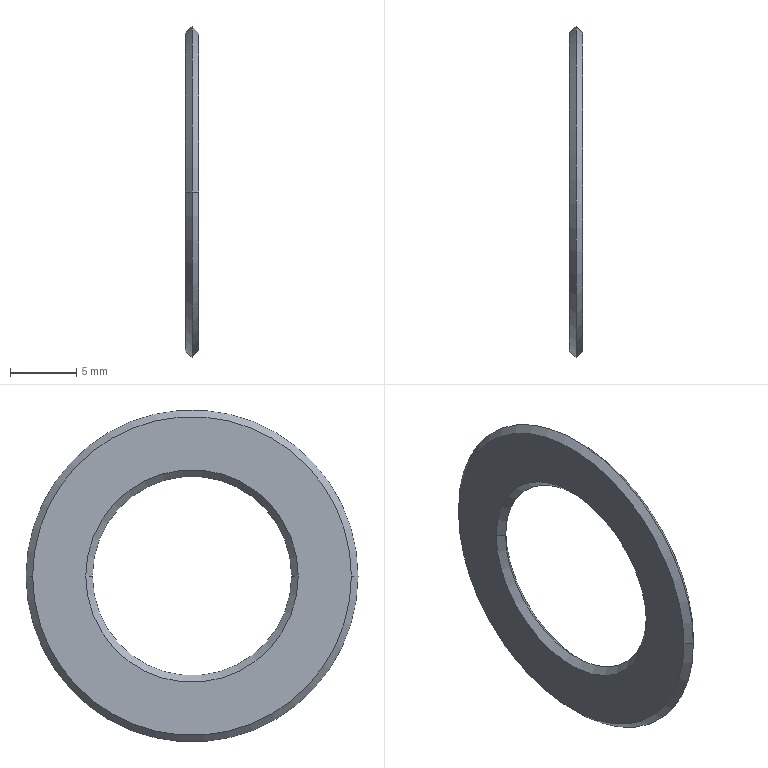Part | STEP file | 0217_005_WSSS25-15-1 | 1 solid | 10 faces | box 1 x 25 x 25 mm | volume 282.743 mm3 | cone 8 | plane 2
STEP:
#1=CARTESIAN_POINT('',(0.,0.,0.));
#2=DIRECTION('',(0.,0.,1.));
#3=DIRECTION('',(1.,0.,0.));
#4=AXIS2_PLACEMENT_3D('',#1,#2,#3);
#5=CARTESIAN_POINT('',(1.,12.,0.));
#6=VERTEX_POINT('',#5);
#7=CARTESIAN_POINT('',(1.,-12.,0.));
#8=VERTEX_POINT('',#7);
#9=CARTESIAN_POINT('',(1.,0.,0.));
#10=DIRECTION('',(1.,0.,0.));
#11=DIRECTION('',(0.,-1.,0.));
#12=AXIS2_PLACEMENT_3D('',#9,#10,#11);
#13=CIRCLE('',#12,12.);
#14=CARTESIAN_POINT('',(0.5,0.,0.));
#15=DIRECTION('',(-1.,0.,0.));
#16=DIRECTION('',(0.,-1.,0.));
#17=AXIS2_PLACEMENT_3D('',#14,#15,#16);
#18=CONICAL_SURFACE('',#17,12.5,0.7854);
#19=CARTESIAN_POINT('',(6.283,-0.5));
#20=DIRECTION('',(-1.,0.));
#21=VECTOR('',#20,1.);
#22=LINE('',#19,#21);
#23=(GEOMETRIC_REPRESENTATION_CONTEXT(2)PARAMETRIC_REPRESENTATION_CONTEXT()REPRESENTATION_CONTEXT('',''));
#24=DEFINITIONAL_REPRESENTATION('',(#22),#23);
#25=PCURVE('',#18,#24);
#26=CARTESIAN_POINT('',(1.,-10.,0.));
#27=DIRECTION('',(1.,0.,0.));
#28=DIRECTION('',(0.,1.,0.));
#29=AXIS2_PLACEMENT_3D('',#26,#27,#28);
#30=PLANE('',#29);
#31=CARTESIAN_POINT('',(10.,0.));
#32=DIRECTION('',(-1.,0.));
#33=AXIS2_PLACEMENT_2D('',#31,#32);
#34=CIRCLE('',#33,12.);
#35=(GEOMETRIC_REPRESENTATION_CONTEXT(2)PARAMETRIC_REPRESENTATION_CONTEXT()REPRESENTATION_CONTEXT('',''));
#36=DEFINITIONAL_REPRESENTATION('',(#34),#35);
#37=PCURVE('',#30,#36);
#38=SURFACE_CURVE('',#13,(#25,#37),.PCURVE_S1.);
#39=EDGE_CURVE('',#6,#8,#38,.T.);
#40=ORIENTED_EDGE('',*,*,#39,.F.);
#41=CARTESIAN_POINT('',(0.5,12.5,0.));
#42=VERTEX_POINT('',#41);
#43=CARTESIAN_POINT('',(0.5,12.5,0.));
#44=DIRECTION('',(-0.7071,0.7071,0.));
#45=VECTOR('',#44,1.);
#46=LINE('',#43,#45);
#47=CARTESIAN_POINT('',(3.142,0.));
#48=DIRECTION('',(0.,1.));
#49=VECTOR('',#48,1.);
#50=LINE('',#47,#49);
#51=(GEOMETRIC_REPRESENTATION_CONTEXT(2)PARAMETRIC_REPRESENTATION_CONTEXT()REPRESENTATION_CONTEXT('',''));
#52=DEFINITIONAL_REPRESENTATION('',(#50),#51);
#53=PCURVE('',#18,#52);
#54=CARTESIAN_POINT('',(0.5,0.,0.));
#55=DIRECTION('',(-1.,0.,0.));
#56=DIRECTION('',(0.,-1.,0.));
#57=AXIS2_PLACEMENT_3D('',#54,#55,#56);
#58=CONICAL_SURFACE('',#57,12.5,0.7854);
#59=CARTESIAN_POINT('',(3.142,0.));
#60=DIRECTION('',(0.,1.));
#61=VECTOR('',#60,1.);
#62=LINE('',#59,#61);
#63=(GEOMETRIC_REPRESENTATION_CONTEXT(2)PARAMETRIC_REPRESENTATION_CONTEXT()REPRESENTATION_CONTEXT('',''));
#64=DEFINITIONAL_REPRESENTATION('',(#62),#63);
#65=PCURVE('',#58,#64);
#66=SURFACE_CURVE('',#46,(#53,#65),.PCURVE_S1.);
#67=EDGE_CURVE('',#6,#42,#66,.T.);
#68=ORIENTED_EDGE('',*,*,#67,.T.);
#69=CARTESIAN_POINT('',(0.5,-12.5,0.));
#70=VERTEX_POINT('',#69);
#71=CARTESIAN_POINT('',(0.5,0.,0.));
#72=DIRECTION('',(1.,0.,0.));
#73=DIRECTION('',(0.,-1.,0.));
#74=AXIS2_PLACEMENT_3D('',#71,#72,#73);
#75=CIRCLE('',#74,12.5);
#76=CARTESIAN_POINT('',(6.283,0.));
#77=DIRECTION('',(-1.,0.));
#78=VECTOR('',#77,1.);
#79=LINE('',#76,#78);
#80=(GEOMETRIC_REPRESENTATION_CONTEXT(2)PARAMETRIC_REPRESENTATION_CONTEXT()REPRESENTATION_CONTEXT('',''));
#81=DEFINITIONAL_REPRESENTATION('',(#79),#80);
#82=PCURVE('',#18,#81);
#83=CARTESIAN_POINT('',(0.5,0.,0.));
#84=DIRECTION('',(1.,0.,0.));
#85=DIRECTION('',(0.,1.,0.));
#86=AXIS2_PLACEMENT_3D('',#83,#84,#85);
#87=CONICAL_SURFACE('',#86,12.5,0.7854);
#88=CARTESIAN_POINT('',(-3.142,0.));
#89=DIRECTION('',(1.,0.));
#90=VECTOR('',#89,1.);
#91=LINE('',#88,#90);
#92=(GEOMETRIC_REPRESENTATION_CONTEXT(2)PARAMETRIC_REPRESENTATION_CONTEXT()REPRESENTATION_CONTEXT('',''));
#93=DEFINITIONAL_REPRESENTATION('',(#91),#92);
#94=PCURVE('',#87,#93);
#95=SURFACE_CURVE('',#75,(#82,#94),.PCURVE_S1.);
#96=EDGE_CURVE('',#42,#70,#95,.T.);
#97=ORIENTED_EDGE('',*,*,#96,.T.);
#98=CARTESIAN_POINT('',(0.5,-12.5,0.));
#99=DIRECTION('',(-0.7071,-0.7071,0.));
#100=VECTOR('',#99,1.);
#101=LINE('',#98,#100);
#102=CARTESIAN_POINT('',(0.,0.));
#103=DIRECTION('',(0.,1.));
#104=VECTOR('',#103,1.);
#105=LINE('',#102,#104);
#106=(GEOMETRIC_REPRESENTATION_CONTEXT(2)PARAMETRIC_REPRESENTATION_CONTEXT()REPRESENTATION_CONTEXT('',''));
#107=DEFINITIONAL_REPRESENTATION('',(#105),#106);
#108=PCURVE('',#18,#107);
#109=CARTESIAN_POINT('',(6.283,0.));
#110=DIRECTION('',(0.,1.));
#111=VECTOR('',#110,1.);
#112=LINE('',#109,#111);
#113=(GEOMETRIC_REPRESENTATION_CONTEXT(2)PARAMETRIC_REPRESENTATION_CONTEXT()REPRESENTATION_CONTEXT('',''));
#114=DEFINITIONAL_REPRESENTATION('',(#112),#113);
#115=PCURVE('',#58,#114);
#116=SURFACE_CURVE('',#101,(#108,#115),.PCURVE_S1.);
#117=EDGE_CURVE('',#8,#70,#116,.T.);
#118=ORIENTED_EDGE('',*,*,#117,.F.);
#119=EDGE_LOOP('',(#40,#68,#97,#118));
#120=FACE_BOUND('',#119,.T.);
#121=ADVANCED_FACE('',(#120),#18,.T.);
#122=CARTESIAN_POINT('',(0.5,7.5,0.));
#123=VERTEX_POINT('',#122);
#124=CARTESIAN_POINT('',(1.,8.,0.));
#125=VERTEX_POINT('',#124);
#126=CARTESIAN_POINT('',(1.,8.,0.));
#127=DIRECTION('',(0.7071,0.7071,0.));
#128=VECTOR('',#127,1.);
#129=LINE('',#126,#128);
#130=CARTESIAN_POINT('',(1.,0.,0.));
#131=DIRECTION('',(1.,0.,0.));
#132=DIRECTION('',(0.,1.,0.));
#133=AXIS2_PLACEMENT_3D('',#130,#131,#132);
#134=CONICAL_SURFACE('',#133,8.,0.7854);
#135=CARTESIAN_POINT('',(6.283,0.));
#136=DIRECTION('',(0.,1.));
#137=VECTOR('',#136,1.);
#138=LINE('',#135,#137);
#139=(GEOMETRIC_REPRESENTATION_CONTEXT(2)PARAMETRIC_REPRESENTATION_CONTEXT()REPRESENTATION_CONTEXT('',''));
#140=DEFINITIONAL_REPRESENTATION('',(#138),#139);
#141=PCURVE('',#134,#140);
#142=CARTESIAN_POINT('',(1.,0.,0.));
#143=DIRECTION('',(1.,0.,0.));
#144=DIRECTION('',(0.,1.,0.));
#145=AXIS2_PLACEMENT_3D('',#142,#143,#144);
#146=CONICAL_SURFACE('',#145,8.,0.7854);
#147=CARTESIAN_POINT('',(0.,0.));
#148=DIRECTION('',(0.,1.));
#149=VECTOR('',#148,1.);
#150=LINE('',#147,#149);
#151=(GEOMETRIC_REPRESENTATION_CONTEXT(2)PARAMETRIC_REPRESENTATION_CONTEXT()REPRESENTATION_CONTEXT('',''));
#152=DEFINITIONAL_REPRESENTATION('',(#150),#151);
#153=PCURVE('',#146,#152);
#154=SURFACE_CURVE('',#129,(#141,#153),.PCURVE_S1.);
#155=EDGE_CURVE('',#123,#125,#154,.T.);
#156=ORIENTED_EDGE('',*,*,#155,.T.);
#157=CARTESIAN_POINT('',(1.,-8.,0.));
#158=VERTEX_POINT('',#157);
#159=CARTESIAN_POINT('',(1.,0.,0.));
#160=DIRECTION('',(-1.,0.,0.));
#161=DIRECTION('',(0.,1.,0.));
#162=AXIS2_PLACEMENT_3D('',#159,#160,#161);
#163=CIRCLE('',#162,8.);
#164=CARTESIAN_POINT('',(6.283,0.));
#165=DIRECTION('',(-1.,0.));
#166=VECTOR('',#165,1.);
#167=LINE('',#164,#166);
#168=(GEOMETRIC_REPRESENTATION_CONTEXT(2)PARAMETRIC_REPRESENTATION_CONTEXT()REPRESENTATION_CONTEXT('',''));
#169=DEFINITIONAL_REPRESENTATION('',(#167),#168);
#170=PCURVE('',#134,#169);
#171=CARTESIAN_POINT('',(18.,0.));
#172=CARTESIAN_POINT('',(18.,-13.856));
#173=CARTESIAN_POINT('',(6.,-6.928));
#174=CARTESIAN_POINT('',(-6.,0.));
#175=CARTESIAN_POINT('',(6.,6.928));
#176=CARTESIAN_POINT('',(18.,13.856));
#177=CARTESIAN_POINT('',(18.,0.));
#178=(BOUNDED_CURVE()B_SPLINE_CURVE(2,(#171,#172,#173,#174,#175,#176,#177),.UNSPECIFIED.,.T.,.F.)B_SPLINE_CURVE_WITH_KNOTS((1,2,2,2,2,1),(-2.094,0.,2.094,4.189,6.283,8.378),.UNSPECIFIED.)CURVE()GEOMETRIC_REPRESENTATION_ITEM()RATIONAL_B_SPLINE_CURVE((1.,0.5,1.,0.5,1.,0.5,1.))REPRESENTATION_ITEM(''));
#179=(GEOMETRIC_REPRESENTATION_CONTEXT(2)PARAMETRIC_REPRESENTATION_CONTEXT()REPRESENTATION_CONTEXT('',''));
#180=DEFINITIONAL_REPRESENTATION('',(#178),#179);
#181=PCURVE('',#30,#180);
#182=SURFACE_CURVE('',#163,(#170,#181),.PCURVE_S1.);
#183=EDGE_CURVE('',#125,#158,#182,.T.);
#184=ORIENTED_EDGE('',*,*,#183,.T.);
#185=CARTESIAN_POINT('',(0.5,-7.5,0.));
#186=VERTEX_POINT('',#185);
#187=CARTESIAN_POINT('',(1.,-8.,0.));
#188=DIRECTION('',(0.7071,-0.7071,0.));
#189=VECTOR('',#188,1.);
#190=LINE('',#187,#189);
#191=CARTESIAN_POINT('',(3.142,0.));
#192=DIRECTION('',(0.,1.));
#193=VECTOR('',#192,1.);
#194=LINE('',#191,#193);
#195=(GEOMETRIC_REPRESENTATION_CONTEXT(2)PARAMETRIC_REPRESENTATION_CONTEXT()REPRESENTATION_CONTEXT('',''));
#196=DEFINITIONAL_REPRESENTATION('',(#194),#195);
#197=PCURVE('',#134,#196);
#198=CARTESIAN_POINT('',(3.142,0.));
#199=DIRECTION('',(0.,1.));
#200=VECTOR('',#199,1.);
#201=LINE('',#198,#200);
#202=(GEOMETRIC_REPRESENTATION_CONTEXT(2)PARAMETRIC_REPRESENTATION_CONTEXT()REPRESENTATION_CONTEXT('',''));
#203=DEFINITIONAL_REPRESENTATION('',(#201),#202);
#204=PCURVE('',#146,#203);
#205=SURFACE_CURVE('',#190,(#197,#204),.PCURVE_S1.);
#206=EDGE_CURVE('',#186,#158,#205,.T.);
#207=ORIENTED_EDGE('',*,*,#206,.F.);
#208=CARTESIAN_POINT('',(0.5,0.,0.));
#209=DIRECTION('',(1.,0.,0.));
#210=DIRECTION('',(0.,-1.,0.));
#211=AXIS2_PLACEMENT_3D('',#208,#209,#210);
#212=CIRCLE('',#211,7.5);
#213=CARTESIAN_POINT('',(3.142,-0.5));
#214=DIRECTION('',(1.,0.));
#215=VECTOR('',#214,1.);
#216=LINE('',#213,#215);
#217=(GEOMETRIC_REPRESENTATION_CONTEXT(2)PARAMETRIC_REPRESENTATION_CONTEXT()REPRESENTATION_CONTEXT('',''));
#218=DEFINITIONAL_REPRESENTATION('',(#216),#217);
#219=PCURVE('',#134,#218);
#220=CARTESIAN_POINT('',(0.,0.,0.));
#221=DIRECTION('',(-1.,0.,0.));
#222=DIRECTION('',(0.,-1.,0.));
#223=AXIS2_PLACEMENT_3D('',#220,#221,#222);
#224=CONICAL_SURFACE('',#223,8.,0.7854);
#225=CARTESIAN_POINT('',(6.283,-0.5));
#226=DIRECTION('',(-1.,0.));
#227=VECTOR('',#226,1.);
#228=LINE('',#225,#227);
#229=(GEOMETRIC_REPRESENTATION_CONTEXT(2)PARAMETRIC_REPRESENTATION_CONTEXT()REPRESENTATION_CONTEXT('',''));
#230=DEFINITIONAL_REPRESENTATION('',(#228),#229);
#231=PCURVE('',#224,#230);
#232=SURFACE_CURVE('',#212,(#219,#231),.PCURVE_S1.);
#233=EDGE_CURVE('',#186,#123,#232,.T.);
#234=ORIENTED_EDGE('',*,*,#233,.T.);
#235=EDGE_LOOP('',(#156,#184,#207,#234));
#236=FACE_BOUND('',#235,.F.);
#237=ADVANCED_FACE('',(#236),#134,.F.);
#238=CARTESIAN_POINT('',(0.,12.,0.));
#239=VERTEX_POINT('',#238);
#240=CARTESIAN_POINT('',(0.,-12.,0.));
#241=VERTEX_POINT('',#240);
#242=CARTESIAN_POINT('',(0.,0.,0.));
#243=DIRECTION('',(1.,0.,0.));
#244=DIRECTION('',(0.,1.,0.));
#245=AXIS2_PLACEMENT_3D('',#242,#243,#244);
#246=CIRCLE('',#245,12.);
#247=CARTESIAN_POINT('',(0.,-0.5));
#248=DIRECTION('',(1.,0.));
#249=VECTOR('',#248,1.);
#250=LINE('',#247,#249);
#251=(GEOMETRIC_REPRESENTATION_CONTEXT(2)PARAMETRIC_REPRESENTATION_CONTEXT()REPRESENTATION_CONTEXT('',''));
#252=DEFINITIONAL_REPRESENTATION('',(#250),#251);
#253=PCURVE('',#87,#252);
#254=CARTESIAN_POINT('',(0.,-10.,0.));
#255=DIRECTION('',(-1.,0.,0.));
#256=DIRECTION('',(0.,-1.,0.));
#257=AXIS2_PLACEMENT_3D('',#254,#255,#256);
#258=PLANE('',#257);
#259=CARTESIAN_POINT('',(-22.,0.));
#260=CARTESIAN_POINT('',(-22.,20.785));
#261=CARTESIAN_POINT('',(-4.,10.392));
#262=CARTESIAN_POINT('',(14.,0.));
#263=CARTESIAN_POINT('',(-4.,-10.392));
#264=CARTESIAN_POINT('',(-22.,-20.785));
#265=CARTESIAN_POINT('',(-22.,0.));
#266=(BOUNDED_CURVE()B_SPLINE_CURVE(2,(#259,#260,#261,#262,#263,#264,#265),.UNSPECIFIED.,.T.,.F.)B_SPLINE_CURVE_WITH_KNOTS((1,2,2,2,2,1),(-2.094,0.,2.094,4.189,6.283,8.378),.UNSPECIFIED.)CURVE()GEOMETRIC_REPRESENTATION_ITEM()RATIONAL_B_SPLINE_CURVE((1.,0.5,1.,0.5,1.,0.5,1.))REPRESENTATION_ITEM(''));
#267=(GEOMETRIC_REPRESENTATION_CONTEXT(2)PARAMETRIC_REPRESENTATION_CONTEXT()REPRESENTATION_CONTEXT('',''));
#268=DEFINITIONAL_REPRESENTATION('',(#266),#267);
#269=PCURVE('',#258,#268);
#270=SURFACE_CURVE('',#246,(#253,#269),.PCURVE_S1.);
#271=EDGE_CURVE('',#239,#241,#270,.T.);
#272=ORIENTED_EDGE('',*,*,#271,.T.);
#273=CARTESIAN_POINT('',(0.5,-12.5,0.));
#274=DIRECTION('',(0.7071,-0.7071,0.));
#275=VECTOR('',#274,1.);
#276=LINE('',#273,#275);
#277=CARTESIAN_POINT('',(3.142,0.));
#278=DIRECTION('',(0.,1.));
#279=VECTOR('',#278,1.);
#280=LINE('',#277,#279);
#281=(GEOMETRIC_REPRESENTATION_CONTEXT(2)PARAMETRIC_REPRESENTATION_CONTEXT()REPRESENTATION_CONTEXT('',''));
#282=DEFINITIONAL_REPRESENTATION('',(#280),#281);
#283=PCURVE('',#87,#282);
#284=CARTESIAN_POINT('',(0.5,0.,0.));
#285=DIRECTION('',(1.,0.,0.));
#286=DIRECTION('',(0.,1.,0.));
#287=AXIS2_PLACEMENT_3D('',#284,#285,#286);
#288=CONICAL_SURFACE('',#287,12.5,0.7854);
#289=CARTESIAN_POINT('',(3.142,0.));
#290=DIRECTION('',(0.,1.));
#291=VECTOR('',#290,1.);
#292=LINE('',#289,#291);
#293=(GEOMETRIC_REPRESENTATION_CONTEXT(2)PARAMETRIC_REPRESENTATION_CONTEXT()REPRESENTATION_CONTEXT('',''));
#294=DEFINITIONAL_REPRESENTATION('',(#292),#293);
#295=PCURVE('',#288,#294);
#296=SURFACE_CURVE('',#276,(#283,#295),.PCURVE_S1.);
#297=EDGE_CURVE('',#241,#70,#296,.T.);
#298=ORIENTED_EDGE('',*,*,#297,.T.);
#299=ORIENTED_EDGE('',*,*,#96,.F.);
#300=CARTESIAN_POINT('',(0.5,12.5,0.));
#301=DIRECTION('',(0.7071,0.7071,0.));
#302=VECTOR('',#301,1.);
#303=LINE('',#300,#302);
#304=CARTESIAN_POINT('',(0.,0.));
#305=DIRECTION('',(0.,1.));
#306=VECTOR('',#305,1.);
#307=LINE('',#304,#306);
#308=(GEOMETRIC_REPRESENTATION_CONTEXT(2)PARAMETRIC_REPRESENTATION_CONTEXT()REPRESENTATION_CONTEXT('',''));
#309=DEFINITIONAL_REPRESENTATION('',(#307),#308);
#310=PCURVE('',#87,#309);
#311=CARTESIAN_POINT('',(6.283,0.));
#312=DIRECTION('',(0.,1.));
#313=VECTOR('',#312,1.);
#314=LINE('',#311,#313);
#315=(GEOMETRIC_REPRESENTATION_CONTEXT(2)PARAMETRIC_REPRESENTATION_CONTEXT()REPRESENTATION_CONTEXT('',''));
#316=DEFINITIONAL_REPRESENTATION('',(#314),#315);
#317=PCURVE('',#288,#316);
#318=SURFACE_CURVE('',#303,(#310,#317),.PCURVE_S1.);
#319=EDGE_CURVE('',#239,#42,#318,.T.);
#320=ORIENTED_EDGE('',*,*,#319,.F.);
#321=EDGE_LOOP('',(#272,#298,#299,#320));
#322=FACE_BOUND('',#321,.T.);
#323=ADVANCED_FACE('',(#322),#87,.T.);
#324=CARTESIAN_POINT('',(0.,-8.,0.));
#325=VERTEX_POINT('',#324);
#326=CARTESIAN_POINT('',(0.,-8.,0.));
#327=DIRECTION('',(-0.7071,-0.7071,0.));
#328=VECTOR('',#327,1.);
#329=LINE('',#326,#328);
#330=CARTESIAN_POINT('',(6.283,0.));
#331=DIRECTION('',(0.,1.));
#332=VECTOR('',#331,1.);
#333=LINE('',#330,#332);
#334=(GEOMETRIC_REPRESENTATION_CONTEXT(2)PARAMETRIC_REPRESENTATION_CONTEXT()REPRESENTATION_CONTEXT('',''));
#335=DEFINITIONAL_REPRESENTATION('',(#333),#334);
#336=PCURVE('',#224,#335);
#337=CARTESIAN_POINT('',(0.,0.,0.));
#338=DIRECTION('',(-1.,0.,0.));
#339=DIRECTION('',(0.,-1.,0.));
#340=AXIS2_PLACEMENT_3D('',#337,#338,#339);
#341=CONICAL_SURFACE('',#340,8.,0.7854);
#342=CARTESIAN_POINT('',(0.,0.));
#343=DIRECTION('',(0.,1.));
#344=VECTOR('',#343,1.);
#345=LINE('',#342,#344);
#346=(GEOMETRIC_REPRESENTATION_CONTEXT(2)PARAMETRIC_REPRESENTATION_CONTEXT()REPRESENTATION_CONTEXT('',''));
#347=DEFINITIONAL_REPRESENTATION('',(#345),#346);
#348=PCURVE('',#341,#347);
#349=SURFACE_CURVE('',#329,(#336,#348),.PCURVE_S1.);
#350=EDGE_CURVE('',#186,#325,#349,.T.);
#351=ORIENTED_EDGE('',*,*,#350,.T.);
#352=CARTESIAN_POINT('',(0.,8.,0.));
#353=VERTEX_POINT('',#352);
#354=CARTESIAN_POINT('',(0.,0.,0.));
#355=DIRECTION('',(1.,0.,0.));
#356=DIRECTION('',(0.,-1.,0.));
#357=AXIS2_PLACEMENT_3D('',#354,#355,#356);
#358=CIRCLE('',#357,8.);
#359=CARTESIAN_POINT('',(6.283,0.));
#360=DIRECTION('',(-1.,0.));
#361=VECTOR('',#360,1.);
#362=LINE('',#359,#361);
#363=(GEOMETRIC_REPRESENTATION_CONTEXT(2)PARAMETRIC_REPRESENTATION_CONTEXT()REPRESENTATION_CONTEXT('',''));
#364=DEFINITIONAL_REPRESENTATION('',(#362),#363);
#365=PCURVE('',#224,#364);
#366=CARTESIAN_POINT('',(-2.,0.));
#367=CARTESIAN_POINT('',(-2.,-13.856));
#368=CARTESIAN_POINT('',(-14.,-6.928));
#369=CARTESIAN_POINT('',(-26.,0.));
#370=CARTESIAN_POINT('',(-14.,6.928));
#371=CARTESIAN_POINT('',(-2.,13.856));
#372=CARTESIAN_POINT('',(-2.,0.));
#373=(BOUNDED_CURVE()B_SPLINE_CURVE(2,(#366,#367,#368,#369,#370,#371,#372),.UNSPECIFIED.,.T.,.F.)B_SPLINE_CURVE_WITH_KNOTS((1,2,2,2,2,1),(-2.094,0.,2.094,4.189,6.283,8.378),.UNSPECIFIED.)CURVE()GEOMETRIC_REPRESENTATION_ITEM()RATIONAL_B_SPLINE_CURVE((1.,0.5,1.,0.5,1.,0.5,1.))REPRESENTATION_ITEM(''));
#374=(GEOMETRIC_REPRESENTATION_CONTEXT(2)PARAMETRIC_REPRESENTATION_CONTEXT()REPRESENTATION_CONTEXT('',''));
#375=DEFINITIONAL_REPRESENTATION('',(#373),#374);
#376=PCURVE('',#258,#375);
#377=SURFACE_CURVE('',#358,(#365,#376),.PCURVE_S1.);
#378=EDGE_CURVE('',#325,#353,#377,.T.);
#379=ORIENTED_EDGE('',*,*,#378,.T.);
#380=CARTESIAN_POINT('',(0.,8.,0.));
#381=DIRECTION('',(-0.7071,0.7071,0.));
#382=VECTOR('',#381,1.);
#383=LINE('',#380,#382);
#384=CARTESIAN_POINT('',(3.142,0.));
#385=DIRECTION('',(0.,1.));
#386=VECTOR('',#385,1.);
#387=LINE('',#384,#386);
#388=(GEOMETRIC_REPRESENTATION_CONTEXT(2)PARAMETRIC_REPRESENTATION_CONTEXT()REPRESENTATION_CONTEXT('',''));
#389=DEFINITIONAL_REPRESENTATION('',(#387),#388);
#390=PCURVE('',#224,#389);
#391=CARTESIAN_POINT('',(3.142,0.));
#392=DIRECTION('',(0.,1.));
#393=VECTOR('',#392,1.);
#394=LINE('',#391,#393);
#395=(GEOMETRIC_REPRESENTATION_CONTEXT(2)PARAMETRIC_REPRESENTATION_CONTEXT()REPRESENTATION_CONTEXT('',''));
#396=DEFINITIONAL_REPRESENTATION('',(#394),#395);
#397=PCURVE('',#341,#396);
#398=SURFACE_CURVE('',#383,(#390,#397),.PCURVE_S1.);
#399=EDGE_CURVE('',#123,#353,#398,.T.);
#400=ORIENTED_EDGE('',*,*,#399,.F.);
#401=ORIENTED_EDGE('',*,*,#233,.F.);
#402=EDGE_LOOP('',(#351,#379,#400,#401));
#403=FACE_BOUND('',#402,.F.);
#404=ADVANCED_FACE('',(#403),#224,.F.);
#405=CARTESIAN_POINT('',(1.,0.,0.));
#406=DIRECTION('',(1.,0.,0.));
#407=DIRECTION('',(0.,-1.,0.));
#408=AXIS2_PLACEMENT_3D('',#405,#406,#407);
#409=CIRCLE('',#408,12.);
#410=CARTESIAN_POINT('',(10.,0.));
#411=DIRECTION('',(-1.,0.));
#412=AXIS2_PLACEMENT_2D('',#410,#411);
#413=CIRCLE('',#412,12.);
#414=(GEOMETRIC_REPRESENTATION_CONTEXT(2)PARAMETRIC_REPRESENTATION_CONTEXT()REPRESENTATION_CONTEXT('',''));
#415=DEFINITIONAL_REPRESENTATION('',(#413),#414);
#416=PCURVE('',#30,#415);
#417=CARTESIAN_POINT('',(6.283,-0.5));
#418=DIRECTION('',(-1.,0.));
#419=VECTOR('',#418,1.);
#420=LINE('',#417,#419);
#421=(GEOMETRIC_REPRESENTATION_CONTEXT(2)PARAMETRIC_REPRESENTATION_CONTEXT()REPRESENTATION_CONTEXT('',''));
#422=DEFINITIONAL_REPRESENTATION('',(#420),#421);
#423=PCURVE('',#58,#422);
#424=SURFACE_CURVE('',#409,(#416,#423),.PCURVE_S1.);
#425=EDGE_CURVE('',#8,#6,#424,.T.);
#426=ORIENTED_EDGE('',*,*,#425,.T.);
#427=ORIENTED_EDGE('',*,*,#39,.T.);
#428=EDGE_LOOP('',(#426,#427));
#429=FACE_BOUND('',#428,.T.);
#430=ORIENTED_EDGE('',*,*,#183,.T.);
#431=CARTESIAN_POINT('',(1.,0.,0.));
#432=DIRECTION('',(-1.,0.,0.));
#433=DIRECTION('',(0.,1.,0.));
#434=AXIS2_PLACEMENT_3D('',#431,#432,#433);
#435=CIRCLE('',#434,8.);
#436=CARTESIAN_POINT('',(18.,0.));
#437=CARTESIAN_POINT('',(18.,-13.856));
#438=CARTESIAN_POINT('',(6.,-6.928));
#439=CARTESIAN_POINT('',(-6.,0.));
#440=CARTESIAN_POINT('',(6.,6.928));
#441=CARTESIAN_POINT('',(18.,13.856));
#442=CARTESIAN_POINT('',(18.,0.));
#443=(BOUNDED_CURVE()B_SPLINE_CURVE(2,(#436,#437,#438,#439,#440,#441,#442),.UNSPECIFIED.,.T.,.F.)B_SPLINE_CURVE_WITH_KNOTS((1,2,2,2,2,1),(-2.094,0.,2.094,4.189,6.283,8.378),.UNSPECIFIED.)CURVE()GEOMETRIC_REPRESENTATION_ITEM()RATIONAL_B_SPLINE_CURVE((1.,0.5,1.,0.5,1.,0.5,1.))REPRESENTATION_ITEM(''));
#444=(GEOMETRIC_REPRESENTATION_CONTEXT(2)PARAMETRIC_REPRESENTATION_CONTEXT()REPRESENTATION_CONTEXT('',''));
#445=DEFINITIONAL_REPRESENTATION('',(#443),#444);
#446=PCURVE('',#30,#445);
#447=CARTESIAN_POINT('',(6.283,0.));
#448=DIRECTION('',(-1.,0.));
#449=VECTOR('',#448,1.);
#450=LINE('',#447,#449);
#451=(GEOMETRIC_REPRESENTATION_CONTEXT(2)PARAMETRIC_REPRESENTATION_CONTEXT()REPRESENTATION_CONTEXT('',''));
#452=DEFINITIONAL_REPRESENTATION('',(#450),#451);
#453=PCURVE('',#146,#452);
#454=SURFACE_CURVE('',#435,(#446,#453),.PCURVE_S1.);
#455=EDGE_CURVE('',#158,#125,#454,.T.);
#456=ORIENTED_EDGE('',*,*,#455,.T.);
#457=EDGE_LOOP('',(#430,#456));
#458=FACE_BOUND('',#457,.T.);
#459=ADVANCED_FACE('',(#429,#458),#30,.T.);
#460=ORIENTED_EDGE('',*,*,#67,.F.);
#461=ORIENTED_EDGE('',*,*,#425,.F.);
#462=ORIENTED_EDGE('',*,*,#117,.T.);
#463=CARTESIAN_POINT('',(0.5,0.,0.));
#464=DIRECTION('',(1.,0.,0.));
#465=DIRECTION('',(0.,-1.,0.));
#466=AXIS2_PLACEMENT_3D('',#463,#464,#465);
#467=CIRCLE('',#466,12.5);
#468=CARTESIAN_POINT('',(6.283,0.));
#469=DIRECTION('',(-1.,0.));
#470=VECTOR('',#469,1.);
#471=LINE('',#468,#470);
#472=(GEOMETRIC_REPRESENTATION_CONTEXT(2)PARAMETRIC_REPRESENTATION_CONTEXT()REPRESENTATION_CONTEXT('',''));
#473=DEFINITIONAL_REPRESENTATION('',(#471),#472);
#474=PCURVE('',#58,#473);
#475=CARTESIAN_POINT('',(3.142,0.));
#476=DIRECTION('',(1.,0.));
#477=VECTOR('',#476,1.);
#478=LINE('',#475,#477);
#479=(GEOMETRIC_REPRESENTATION_CONTEXT(2)PARAMETRIC_REPRESENTATION_CONTEXT()REPRESENTATION_CONTEXT('',''));
#480=DEFINITIONAL_REPRESENTATION('',(#478),#479);
#481=PCURVE('',#288,#480);
#482=SURFACE_CURVE('',#467,(#474,#481),.PCURVE_S1.);
#483=EDGE_CURVE('',#70,#42,#482,.T.);
#484=ORIENTED_EDGE('',*,*,#483,.T.);
#485=EDGE_LOOP('',(#460,#461,#462,#484));
#486=FACE_BOUND('',#485,.T.);
#487=ADVANCED_FACE('',(#486),#58,.T.);
#488=ORIENTED_EDGE('',*,*,#455,.T.);
#489=ORIENTED_EDGE('',*,*,#155,.F.);
#490=CARTESIAN_POINT('',(0.5,0.,0.));
#491=DIRECTION('',(1.,0.,0.));
#492=DIRECTION('',(0.,-1.,0.));
#493=AXIS2_PLACEMENT_3D('',#490,#491,#492);
#494=CIRCLE('',#493,7.5);
#495=CARTESIAN_POINT('',(-3.142,-0.5));
#496=DIRECTION('',(1.,0.));
#497=VECTOR('',#496,1.);
#498=LINE('',#495,#497);
#499=(GEOMETRIC_REPRESENTATION_CONTEXT(2)PARAMETRIC_REPRESENTATION_CONTEXT()REPRESENTATION_CONTEXT('',''));
#500=DEFINITIONAL_REPRESENTATION('',(#498),#499);
#501=PCURVE('',#146,#500);
#502=CARTESIAN_POINT('',(6.283,-0.5));
#503=DIRECTION('',(-1.,0.));
#504=VECTOR('',#503,1.);
#505=LINE('',#502,#504);
#506=(GEOMETRIC_REPRESENTATION_CONTEXT(2)PARAMETRIC_REPRESENTATION_CONTEXT()REPRESENTATION_CONTEXT('',''));
#507=DEFINITIONAL_REPRESENTATION('',(#505),#506);
#508=PCURVE('',#341,#507);
#509=SURFACE_CURVE('',#494,(#501,#508),.PCURVE_S1.);
#510=EDGE_CURVE('',#123,#186,#509,.T.);
#511=ORIENTED_EDGE('',*,*,#510,.T.);
#512=ORIENTED_EDGE('',*,*,#206,.T.);
#513=EDGE_LOOP('',(#488,#489,#511,#512));
#514=FACE_BOUND('',#513,.F.);
#515=ADVANCED_FACE('',(#514),#146,.F.);
#516=ORIENTED_EDGE('',*,*,#297,.F.);
#517=CARTESIAN_POINT('',(0.,0.,0.));
#518=DIRECTION('',(1.,0.,0.));
#519=DIRECTION('',(0.,1.,0.));
#520=AXIS2_PLACEMENT_3D('',#517,#518,#519);
#521=CIRCLE('',#520,12.);
#522=CARTESIAN_POINT('',(0.,-0.5));
#523=DIRECTION('',(1.,0.));
#524=VECTOR('',#523,1.);
#525=LINE('',#522,#524);
#526=(GEOMETRIC_REPRESENTATION_CONTEXT(2)PARAMETRIC_REPRESENTATION_CONTEXT()REPRESENTATION_CONTEXT('',''));
#527=DEFINITIONAL_REPRESENTATION('',(#525),#526);
#528=PCURVE('',#288,#527);
#529=CARTESIAN_POINT('',(-22.,0.));
#530=CARTESIAN_POINT('',(-22.,20.785));
#531=CARTESIAN_POINT('',(-4.,10.392));
#532=CARTESIAN_POINT('',(14.,0.));
#533=CARTESIAN_POINT('',(-4.,-10.392));
#534=CARTESIAN_POINT('',(-22.,-20.785));
#535=CARTESIAN_POINT('',(-22.,0.));
#536=(BOUNDED_CURVE()B_SPLINE_CURVE(2,(#529,#530,#531,#532,#533,#534,#535),.UNSPECIFIED.,.T.,.F.)B_SPLINE_CURVE_WITH_KNOTS((1,2,2,2,2,1),(-2.094,0.,2.094,4.189,6.283,8.378),.UNSPECIFIED.)CURVE()GEOMETRIC_REPRESENTATION_ITEM()RATIONAL_B_SPLINE_CURVE((1.,0.5,1.,0.5,1.,0.5,1.))REPRESENTATION_ITEM(''));
#537=(GEOMETRIC_REPRESENTATION_CONTEXT(2)PARAMETRIC_REPRESENTATION_CONTEXT()REPRESENTATION_CONTEXT('',''));
#538=DEFINITIONAL_REPRESENTATION('',(#536),#537);
#539=PCURVE('',#258,#538);
#540=SURFACE_CURVE('',#521,(#528,#539),.PCURVE_S1.);
#541=EDGE_CURVE('',#241,#239,#540,.T.);
#542=ORIENTED_EDGE('',*,*,#541,.T.);
#543=ORIENTED_EDGE('',*,*,#319,.T.);
#544=ORIENTED_EDGE('',*,*,#483,.F.);
#545=EDGE_LOOP('',(#516,#542,#543,#544));
#546=FACE_BOUND('',#545,.T.);
#547=ADVANCED_FACE('',(#546),#288,.T.);
#548=CARTESIAN_POINT('',(0.,0.,0.));
#549=DIRECTION('',(1.,0.,0.));
#550=DIRECTION('',(0.,-1.,0.));
#551=AXIS2_PLACEMENT_3D('',#548,#549,#550);
#552=CIRCLE('',#551,8.);
#553=CARTESIAN_POINT('',(6.283,0.));
#554=DIRECTION('',(-1.,0.));
#555=VECTOR('',#554,1.);
#556=LINE('',#553,#555);
#557=(GEOMETRIC_REPRESENTATION_CONTEXT(2)PARAMETRIC_REPRESENTATION_CONTEXT()REPRESENTATION_CONTEXT('',''));
#558=DEFINITIONAL_REPRESENTATION('',(#556),#557);
#559=PCURVE('',#341,#558);
#560=CARTESIAN_POINT('',(-2.,0.));
#561=CARTESIAN_POINT('',(-2.,-13.856));
#562=CARTESIAN_POINT('',(-14.,-6.928));
#563=CARTESIAN_POINT('',(-26.,0.));
#564=CARTESIAN_POINT('',(-14.,6.928));
#565=CARTESIAN_POINT('',(-2.,13.856));
#566=CARTESIAN_POINT('',(-2.,0.));
#567=(BOUNDED_CURVE()B_SPLINE_CURVE(2,(#560,#561,#562,#563,#564,#565,#566),.UNSPECIFIED.,.T.,.F.)B_SPLINE_CURVE_WITH_KNOTS((1,2,2,2,2,1),(-2.094,0.,2.094,4.189,6.283,8.378),.UNSPECIFIED.)CURVE()GEOMETRIC_REPRESENTATION_ITEM()RATIONAL_B_SPLINE_CURVE((1.,0.5,1.,0.5,1.,0.5,1.))REPRESENTATION_ITEM(''));
#568=(GEOMETRIC_REPRESENTATION_CONTEXT(2)PARAMETRIC_REPRESENTATION_CONTEXT()REPRESENTATION_CONTEXT('',''));
#569=DEFINITIONAL_REPRESENTATION('',(#567),#568);
#570=PCURVE('',#258,#569);
#571=SURFACE_CURVE('',#552,(#559,#570),.PCURVE_S1.);
#572=EDGE_CURVE('',#353,#325,#571,.T.);
#573=ORIENTED_EDGE('',*,*,#572,.T.);
#574=ORIENTED_EDGE('',*,*,#350,.F.);
#575=ORIENTED_EDGE('',*,*,#510,.F.);
#576=ORIENTED_EDGE('',*,*,#399,.T.);
#577=EDGE_LOOP('',(#573,#574,#575,#576));
#578=FACE_BOUND('',#577,.F.);
#579=ADVANCED_FACE('',(#578),#341,.F.);
#580=ORIENTED_EDGE('',*,*,#378,.T.);
#581=ORIENTED_EDGE('',*,*,#572,.T.);
#582=EDGE_LOOP('',(#580,#581));
#583=FACE_BOUND('',#582,.T.);
#584=ORIENTED_EDGE('',*,*,#271,.F.);
#585=ORIENTED_EDGE('',*,*,#541,.F.);
#586=EDGE_LOOP('',(#584,#585));
#587=FACE_BOUND('',#586,.T.);
#588=ADVANCED_FACE('',(#583,#587),#258,.T.);
#589=CLOSED_SHELL('',(#121,#237,#323,#404,#459,#487,#515,#547,#579,#588));
#590=MANIFOLD_SOLID_BREP('',#589);
#591=(LENGTH_UNIT()NAMED_UNIT(*)SI_UNIT(.MILLI.,.METRE.));
#592=UNCERTAINTY_MEASURE_WITH_UNIT(LENGTH_MEASURE(0.0000001),#591,'','');
#593=(NAMED_UNIT(*)PLANE_ANGLE_UNIT()SI_UNIT($,.RADIAN.));
#594=(NAMED_UNIT(*)SI_UNIT($,.STERADIAN.)SOLID_ANGLE_UNIT());
#595=(GEOMETRIC_REPRESENTATION_CONTEXT(3)GLOBAL_UNCERTAINTY_ASSIGNED_CONTEXT((#592))GLOBAL_UNIT_ASSIGNED_CONTEXT((#591,#593,#594))REPRESENTATION_CONTEXT('',''));
#596=ADVANCED_BREP_SHAPE_REPRESENTATION('',(#4,#590),#595);